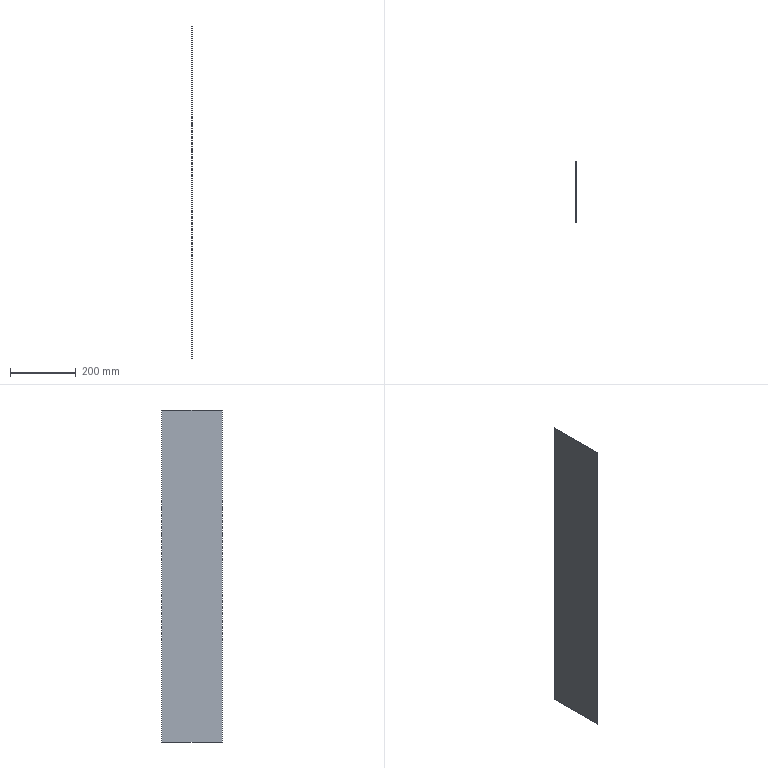Part | SolidWorks | 1 solid | 6 faces | box 1.5 x 185 x 1010 mm | volume 280275 mm3 | plane 6
STEP:
#1=CARTESIAN_POINT('',(0.,92.5,505.));
#2=VERTEX_POINT('',#1);
#3=CARTESIAN_POINT('',(0.,-92.5,505.));
#4=VERTEX_POINT('',#3);
#5=CARTESIAN_POINT('',(0.,-92.5,505.));
#6=DIRECTION('',(0.,-1.,0.));
#7=VECTOR('',#6,1000.);
#8=LINE('',#5,#7);
#9=EDGE_CURVE('',#2,#4,#8,.T.);
#10=ORIENTED_EDGE('',*,*,#9,.F.);
#11=CARTESIAN_POINT('',(-1.5,92.5,505.));
#12=VERTEX_POINT('',#11);
#13=CARTESIAN_POINT('',(-1.5,92.5,505.));
#14=DIRECTION('',(1.,0.,0.));
#15=VECTOR('',#14,1000.);
#16=LINE('',#13,#15);
#17=EDGE_CURVE('',#12,#2,#16,.T.);
#18=ORIENTED_EDGE('',*,*,#17,.F.);
#19=CARTESIAN_POINT('',(-1.5,-92.5,505.));
#20=VERTEX_POINT('',#19);
#21=CARTESIAN_POINT('',(-1.5,-92.5,505.));
#22=DIRECTION('',(0.,-1.,0.));
#23=VECTOR('',#22,1000.);
#24=LINE('',#21,#23);
#25=EDGE_CURVE('',#12,#20,#24,.T.);
#26=ORIENTED_EDGE('',*,*,#25,.T.);
#27=CARTESIAN_POINT('',(-1.5,-92.5,505.));
#28=DIRECTION('',(1.,0.,0.));
#29=VECTOR('',#28,1000.);
#30=LINE('',#27,#29);
#31=EDGE_CURVE('',#20,#4,#30,.T.);
#32=ORIENTED_EDGE('',*,*,#31,.T.);
#33=EDGE_LOOP('',(#10,#18,#26,#32));
#34=FACE_OUTER_BOUND('',#33,.T.);
#35=CARTESIAN_POINT('',(-1.5,-92.5,505.));
#36=DIRECTION('',(0.,0.,1.));
#37=DIRECTION('',(1.,0.,0.));
#38=AXIS2_PLACEMENT_3D('',#35,#36,#37);
#39=PLANE('',#38);
#40=ADVANCED_FACE('',(#34),#39,.T.);
#41=CARTESIAN_POINT('',(0.,92.5,-505.));
#42=VERTEX_POINT('',#41);
#43=CARTESIAN_POINT('',(0.,92.5,-505.));
#44=DIRECTION('',(0.,0.,1.));
#45=VECTOR('',#44,1000.);
#46=LINE('',#43,#45);
#47=EDGE_CURVE('',#42,#2,#46,.T.);
#48=ORIENTED_EDGE('',*,*,#47,.F.);
#49=CARTESIAN_POINT('',(-1.5,92.5,-505.));
#50=VERTEX_POINT('',#49);
#51=CARTESIAN_POINT('',(-1.5,92.5,-505.));
#52=DIRECTION('',(1.,0.,0.));
#53=VECTOR('',#52,1000.);
#54=LINE('',#51,#53);
#55=EDGE_CURVE('',#50,#42,#54,.T.);
#56=ORIENTED_EDGE('',*,*,#55,.F.);
#57=CARTESIAN_POINT('',(-1.5,92.5,-505.));
#58=DIRECTION('',(0.,0.,1.));
#59=VECTOR('',#58,1000.);
#60=LINE('',#57,#59);
#61=EDGE_CURVE('',#50,#12,#60,.T.);
#62=ORIENTED_EDGE('',*,*,#61,.T.);
#63=ORIENTED_EDGE('',*,*,#17,.T.);
#64=EDGE_LOOP('',(#48,#56,#62,#63));
#65=FACE_OUTER_BOUND('',#64,.T.);
#66=CARTESIAN_POINT('',(-1.5,92.5,-505.));
#67=DIRECTION('',(0.,1.,0.));
#68=DIRECTION('',(0.,0.,1.));
#69=AXIS2_PLACEMENT_3D('',#66,#67,#68);
#70=PLANE('',#69);
#71=ADVANCED_FACE('',(#65),#70,.T.);
#72=CARTESIAN_POINT('',(0.,-92.5,-505.));
#73=VERTEX_POINT('',#72);
#74=CARTESIAN_POINT('',(0.,-92.5,-505.));
#75=DIRECTION('',(0.,1.,0.));
#76=VECTOR('',#75,1000.);
#77=LINE('',#74,#76);
#78=EDGE_CURVE('',#73,#42,#77,.T.);
#79=ORIENTED_EDGE('',*,*,#78,.F.);
#80=CARTESIAN_POINT('',(-1.5,-92.5,-505.));
#81=VERTEX_POINT('',#80);
#82=CARTESIAN_POINT('',(-1.5,-92.5,-505.));
#83=DIRECTION('',(1.,0.,0.));
#84=VECTOR('',#83,1000.);
#85=LINE('',#82,#84);
#86=EDGE_CURVE('',#81,#73,#85,.T.);
#87=ORIENTED_EDGE('',*,*,#86,.F.);
#88=CARTESIAN_POINT('',(-1.5,-92.5,-505.));
#89=DIRECTION('',(0.,1.,0.));
#90=VECTOR('',#89,1000.);
#91=LINE('',#88,#90);
#92=EDGE_CURVE('',#81,#50,#91,.T.);
#93=ORIENTED_EDGE('',*,*,#92,.T.);
#94=ORIENTED_EDGE('',*,*,#55,.T.);
#95=EDGE_LOOP('',(#79,#87,#93,#94));
#96=FACE_OUTER_BOUND('',#95,.T.);
#97=CARTESIAN_POINT('',(-1.5,-92.5,-505.));
#98=DIRECTION('',(0.,0.,-1.));
#99=DIRECTION('',(-1.,0.,0.));
#100=AXIS2_PLACEMENT_3D('',#97,#98,#99);
#101=PLANE('',#100);
#102=ADVANCED_FACE('',(#96),#101,.T.);
#103=CARTESIAN_POINT('',(0.,-92.5,-505.));
#104=DIRECTION('',(0.,0.,-1.));
#105=VECTOR('',#104,1000.);
#106=LINE('',#103,#105);
#107=EDGE_CURVE('',#4,#73,#106,.T.);
#108=ORIENTED_EDGE('',*,*,#107,.F.);
#109=ORIENTED_EDGE('',*,*,#31,.F.);
#110=CARTESIAN_POINT('',(-1.5,-92.5,-505.));
#111=DIRECTION('',(0.,0.,-1.));
#112=VECTOR('',#111,1000.);
#113=LINE('',#110,#112);
#114=EDGE_CURVE('',#20,#81,#113,.T.);
#115=ORIENTED_EDGE('',*,*,#114,.T.);
#116=ORIENTED_EDGE('',*,*,#86,.T.);
#117=EDGE_LOOP('',(#108,#109,#115,#116));
#118=FACE_OUTER_BOUND('',#117,.T.);
#119=CARTESIAN_POINT('',(-1.5,-92.5,-505.));
#120=DIRECTION('',(0.,-1.,0.));
#121=DIRECTION('',(0.,0.,-1.));
#122=AXIS2_PLACEMENT_3D('',#119,#120,#121);
#123=PLANE('',#122);
#124=ADVANCED_FACE('',(#118),#123,.T.);
#125=ORIENTED_EDGE('',*,*,#25,.F.);
#126=ORIENTED_EDGE('',*,*,#61,.F.);
#127=ORIENTED_EDGE('',*,*,#92,.F.);
#128=ORIENTED_EDGE('',*,*,#114,.F.);
#129=EDGE_LOOP('',(#125,#126,#127,#128));
#130=FACE_OUTER_BOUND('',#129,.T.);
#131=CARTESIAN_POINT('',(-1.5,0.,0.));
#132=DIRECTION('',(1.,0.,0.));
#133=DIRECTION('',(0.,0.,-1.));
#134=AXIS2_PLACEMENT_3D('',#131,#132,#133);
#135=PLANE('',#134);
#136=ADVANCED_FACE('',(#130),#135,.F.);
#137=ORIENTED_EDGE('',*,*,#9,.T.);
#138=ORIENTED_EDGE('',*,*,#107,.T.);
#139=ORIENTED_EDGE('',*,*,#78,.T.);
#140=ORIENTED_EDGE('',*,*,#47,.T.);
#141=EDGE_LOOP('',(#137,#138,#139,#140));
#142=FACE_OUTER_BOUND('',#141,.T.);
#143=CARTESIAN_POINT('',(0.,0.,0.));
#144=DIRECTION('',(1.,0.,0.));
#145=DIRECTION('',(0.,0.,-1.));
#146=AXIS2_PLACEMENT_3D('',#143,#144,#145);
#147=PLANE('',#146);
#148=ADVANCED_FACE('',(#142),#147,.T.);
#149=CLOSED_SHELL('',(#40,#71,#102,#124,#136,#148));
#150=MANIFOLD_SOLID_BREP('',#149);
#151=CARTESIAN_POINT('',(0.,0.,0.));
#152=DIRECTION('',(0.,0.,1.));
#153=DIRECTION('',(1.,0.,0.));
#154=AXIS2_PLACEMENT_3D('',#151,#152,#153);
#155=(LENGTH_UNIT()NAMED_UNIT(*)SI_UNIT(.MILLI.,.METRE.));
#156=UNCERTAINTY_MEASURE_WITH_UNIT(LENGTH_MEASURE(0.00001),#155,'','');
#157=(NAMED_UNIT(*)PLANE_ANGLE_UNIT()SI_UNIT($,.RADIAN.));
#158=(NAMED_UNIT(*)SI_UNIT($,.STERADIAN.)SOLID_ANGLE_UNIT());
#159=(GEOMETRIC_REPRESENTATION_CONTEXT(3)GLOBAL_UNCERTAINTY_ASSIGNED_CONTEXT((#156))GLOBAL_UNIT_ASSIGNED_CONTEXT((#155,#157,#158))REPRESENTATION_CONTEXT('',''));
#160=ADVANCED_BREP_SHAPE_REPRESENTATION('',(#150,#154),#159);